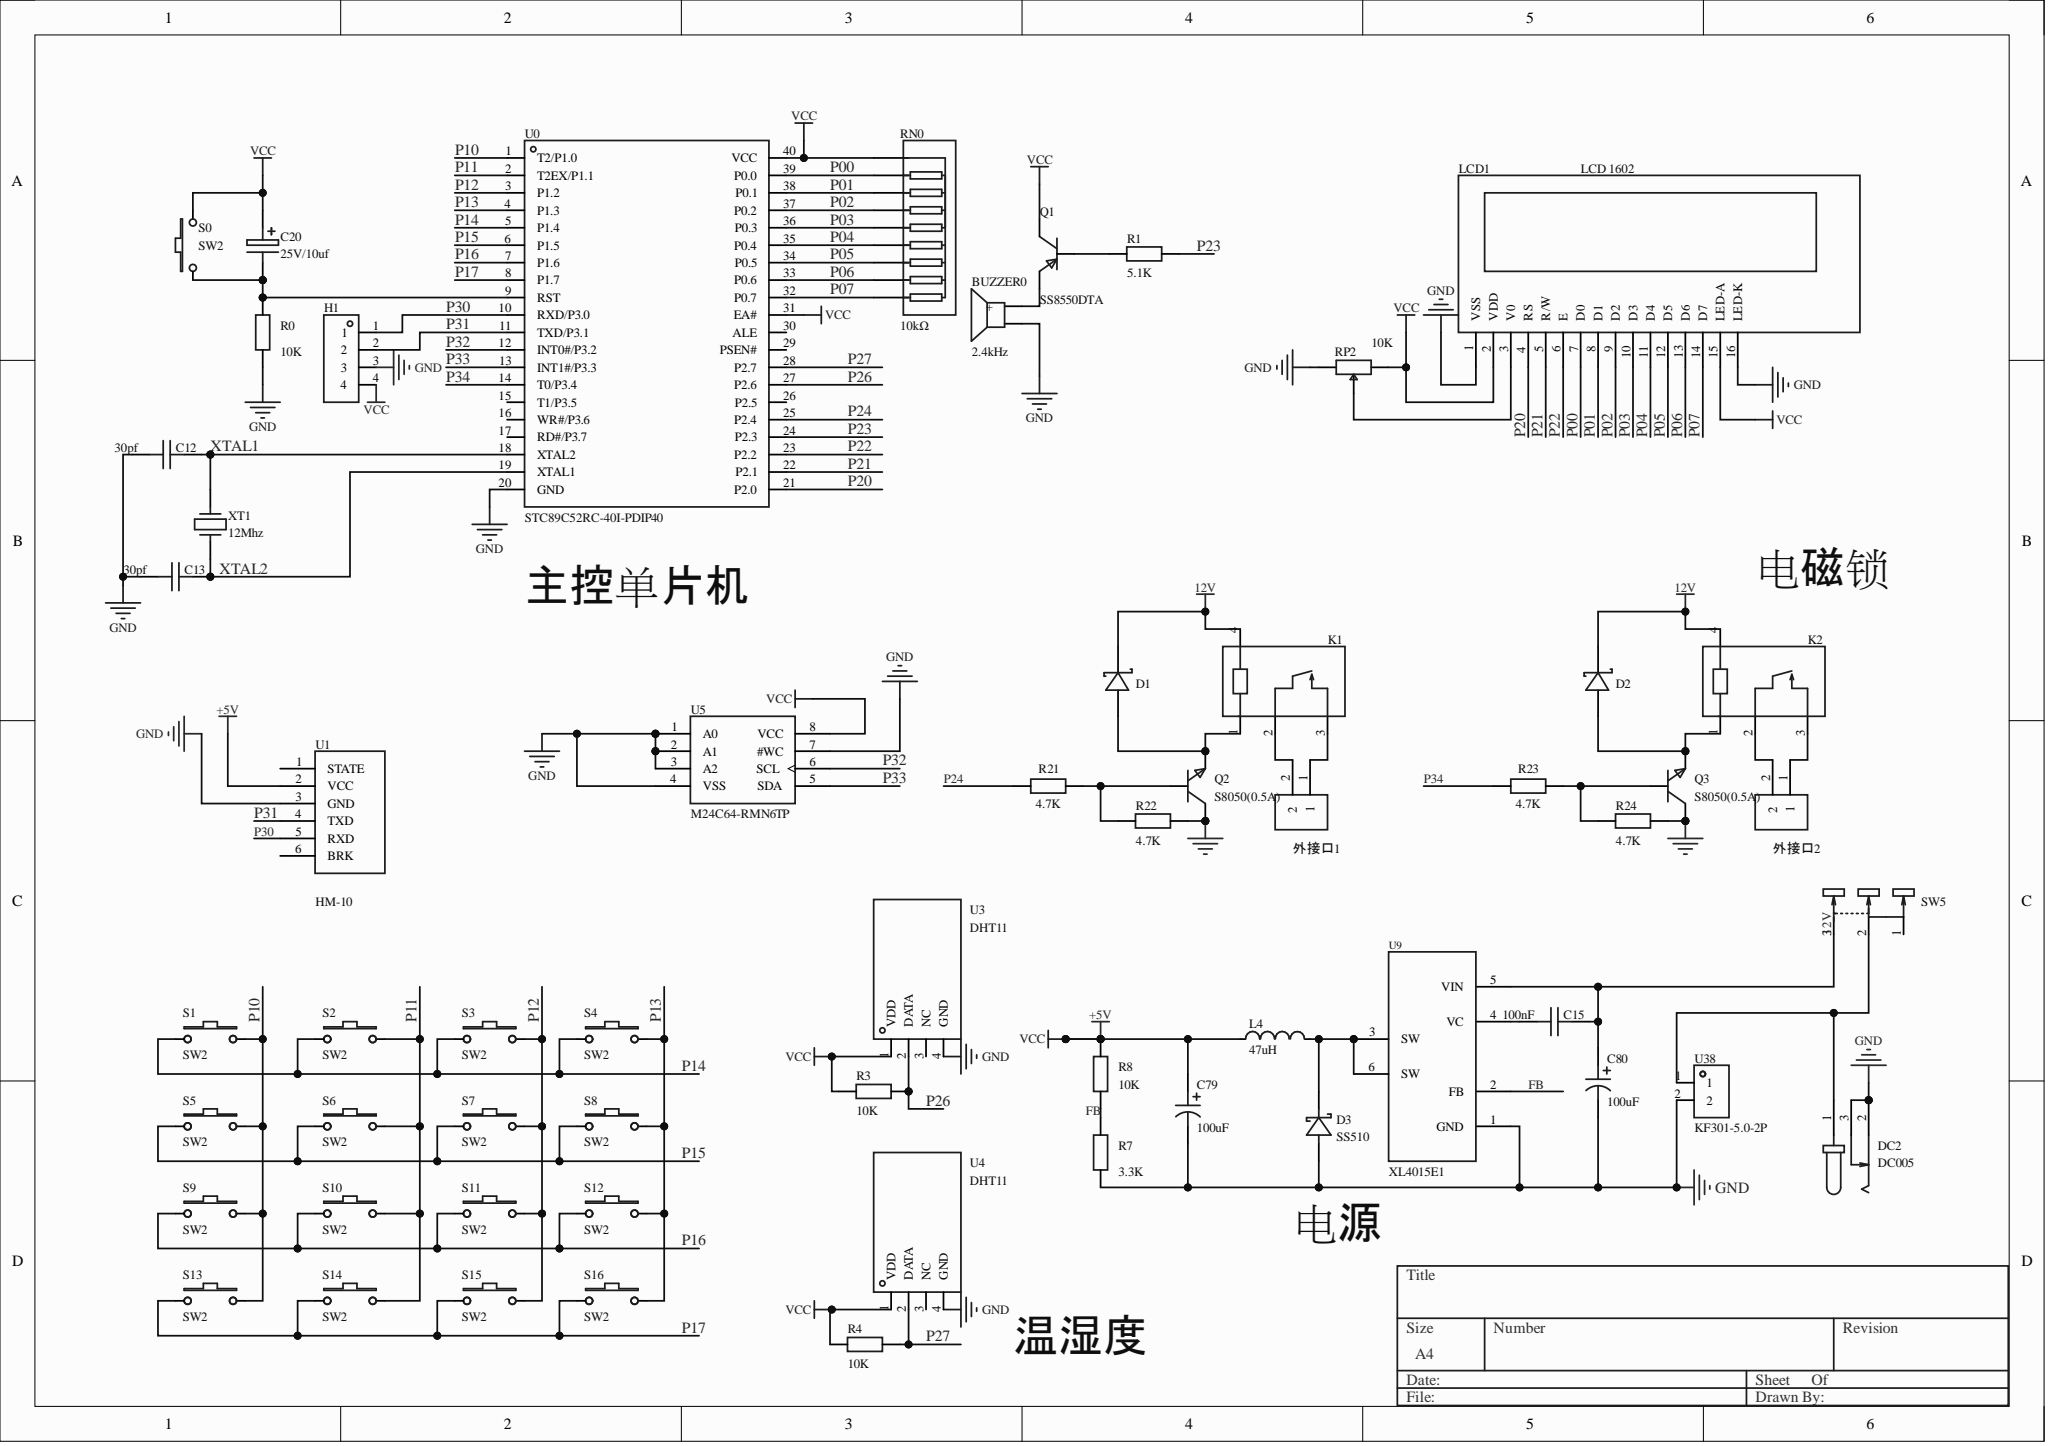Circuit board | Altium Designer | 59 parts | 49 nets
Bill of materials:
Comment,Description,Designator,Footprint,LibRef,Quantity
"2.4kHz","驱动方式:有源(内含驱动线路);构造类型:电磁式;额定电压:5V;频率:2.4kHz;声压(SPL):85dB;","BUZZER0","BUZ-TH_BD12.0-P7.60-D0.6-FD","TMB12A05_C96093","1"
"30pf","","C12, C13","C0805","CAP_0805","2"
"100nF","","C15","C0805","CAP_0805","1"
"CAP-E","","C20","CAP-TH_BD5.0-P2.00-D0.5-FD-A","CAP-E","1"
"100uF","容值:100uF;精度:±20%;额定电压:35V;纹波电流:87mA@120kHz;等效串联电阻:-;","C79, C80","CAP-SMD_BD6.3-L6.6-W6.6-LS7.4-FD","RVT100UF35V67RV0034","2"
"","","D1, D2","SMC_L6.9-W5.9-LS7.9-RD","SS34_C154551","2"
"SS510","二极管配置:独立式;直流反向耐压(Vr):100V;平均整流电流(Io):5A;正向压降(Vf):850mV@5A;","D3","SMA_L4.3-W2.6-LS5.0-RD","SS510_C727067","1"
"DC005","连接器类型:DC电源插座;安装方式:弯插;触点内径:2mm;触点外径:6.3mm;额定电流:500mA;额定电压:12V;工作温度:-30℃~+70℃;","DC2","DC-IN-TH_DC005","DC005","1"
"","","H1","HDR-TH_4P-P2.54-V-F","HDR-F_2.54_1x4P","1"
"","","K1, K2","RELAY-TH_G5NB-1A-E-DCXX","G5NB-1A-E-12VDC","2"
"47uH","类型:屏蔽电感;电感值:47uH;精度:±20%;额定电流:2.5A;饱和电流(Isat):4.6A;","L4","IND-SMD_L12.3-W12.3","SMDRI127-470MT","1"
"LCD 1602","LCD 1602","LCD1","LCD1602","LCD 1602","1"
"SS8550DTA","晶体管类型:PNP;集电极电流(Ic):1.5A;集射极击穿电压(Vceo):25V;耗散功率(Pd):2W;直流电流增益(hFE):40@800mA,1V;","Q1","TO-92-3_L4.8-W3.7-P2.54-L","SS8550DTA","1"
"S8050(0.5A)","晶体管类型:NPN;集电极电流(Ic):500mA;集射极击穿电压(Vceo):25V;耗散功率(Pd):300mW;直流电流增益(hFE):120;","Q2, Q3","SOT-23-3_L2.9-W1.3-P1.90-LS2.4-BR","S8050(0.5A)","2"
"10K","","R0, R3, R4, R8","R0805","Res_0805","4"
"5.1K","","R1","R0805","Res_0805","1"
"3.3K","","R7","R0805","Res_0805","1"
"4.7K","","R21, R22, R23, R24","R0805","Res_0805","4"
"10kΩ","","RN0","RES-ARRAY-TH_9P-P2.54-D1.0","A09-103JP","1"
"10K","","RP2","RES-ADJ-TH_3296W-1-203","10K","1"
"SW2","","S0, S1, S2, S3, S4, S5, S6, S7, S8, S9, S10, S11, S12, S13, S14, S15, S16","SW-SMD_L3.9-W2.9-LS5.0","SW2","17"
"SS-12D10L5","电路结构:单刀双掷;安装方式:直插;开关颜色:黑色;额定电流:3A;额定电压:125V;工作寿命:1万次;","SW5","SW-TH_SS-12D10L5","SS-12D10L5","1"
"STC89C52RC-40I-PDIP40","CPU内核:51家族;CPU最大主频:-;","U0","DIP-40_L52.0-W13.7-P2.54-LS15.2-BL","STC89C52RC-40I-PDIP40","1"
"HM-10","","U1","HM-10.288","hm10","1"
"DHT11","温度范围:-20℃~+60℃;湿度范围:5%RH~95%RH;湿度精度:±5%RH;","U3, U4","SENSOR-TH_DHT11","DHT11","2"
"M24C64-RMN6TP","接口类型:I2C;存储容量:64Kbit;时钟频率(fc):1MHz;","U5","SOIC-8_L5.0-W4.0-P1.27-LS6.0-BL","M24C64-RMN6TP","1"
"XL4015E1","功能类型:降压型;输入电压:-;输出电流(最大值):-;","U9","TO-263-5_L10.2-W8.9-P1.70-TL","XL4015E1","1"
"KF301-5.0-2P","结构:1x2P;间距:5mm;颜色:蓝色;安装方式:直插;额定电流:17A;额定电压:250V;排数:1;线规 - AWG:14~22;线规 - 平方毫米:1.5;每排PIN数:2;工作温度范围:-30℃~+120℃;","U38","CONN-TH_P5.00_KF301-5.0-2P","KF301-5.0-2P","1"
"XT","","XT1","HC-49S_L7.2-W3.2","XT","1"
"","","外接口1, 外接口2","CONN-TH_2P-P5.00_WJ500V-5.08-2P","WJ500V-5.08-2P","2"
Netlist (Protel format):
[
BUZZER0
BUZ-TH_BD12.0-P7.60-D0.6-FD
2.4kHz



]
[
C12
C0805
30pf



]
[
C13
C0805
30pf



]
[
C15
C0805
100nF



]
[
C20
CAP-TH_BD5.0-P2.00-D0.5-FD-A
CAP-E



]
[
C79
CAP-SMD_BD6.3-L6.6-W6.6-LS7.4-FD
100uF



]
[
C80
CAP-SMD_BD6.3-L6.6-W6.6-LS7.4-FD
100uF



]
[
D1
SMC_L6.9-W5.9-LS7.9-RD




]
[
D2
SMC_L6.9-W5.9-LS7.9-RD




]
[
D3
SMA_L4.3-W2.6-LS5.0-RD
SS510



]
[
DC2
DC-IN-TH_DC005
DC005



]
[
H1
HDR-TH_4P-P2.54-V-F




]
[
K1
RELAY-TH_G5NB-1A-E-DCXX




]
[
K2
RELAY-TH_G5NB-1A-E-DCXX




]
[
L4
IND-SMD_L12.3-W12.3
47uH



]
[
LCD1
LCD1602
LCD 1602



]
[
Q1
TO-92-3_L4.8-W3.7-P2.54-L
SS8550DTA



]
[
Q2
SOT-23-3_L2.9-W1.3-P1.90-LS2.4-BR
S8050(0.5A)



]
[
Q3
SOT-23-3_L2.9-W1.3-P1.90-LS2.4-BR
S8050(0.5A)



]
[
R0
R0805
10K



]
[
R1
R0805
5.1K



]
[
R3
R0805
10K



]
[
R4
R0805
10K



]
[
R7
R0805
3.3K



]
[
R8
R0805
10K



]
[
R21
R0805
4.7K



]
[
R22
R0805
4.7K



]
[
R23
R0805
4.7K



]
[
R24
R0805
4.7K



]
[
RN0
RES-ARRAY-TH_9P-P2.54-D1.0
10kΩ



]
[
RP2
RES-ADJ-TH_3296W-1-203
10K



]
[
S0
SW-SMD_L3.9-W2.9-LS5.0
SW2



]
[
S1
SW-SMD_L3.9-W2.9-LS5.0
SW2



]
[
S2
SW-SMD_L3.9-W2.9-LS5.0
SW2



]
[
S3
SW-SMD_L3.9-W2.9-LS5.0
SW2



]
[
S4
SW-SMD_L3.9-W2.9-LS5.0
SW2



]
[
S5
SW-SMD_L3.9-W2.9-LS5.0
SW2



]
[
S6
SW-SMD_L3.9-W2.9-LS5.0
SW2



]
[
S7
SW-SMD_L3.9-W2.9-LS5.0
SW2



]
[
S8
SW-SMD_L3.9-W2.9-LS5.0
SW2



]
[
S9
SW-SMD_L3.9-W2.9-LS5.0
SW2



]
[
S10
SW-SMD_L3.9-W2.9-LS5.0
SW2



]
[
S11
SW-SMD_L3.9-W2.9-LS5.0
SW2



]
[
S12
SW-SMD_L3.9-W2.9-LS5.0
SW2



]
[
S13
SW-SMD_L3.9-W2.9-LS5.0
SW2



]
[
S14
SW-SMD_L3.9-W2.9-LS5.0
SW2



]
[
S15
SW-SMD_L3.9-W2.9-LS5.0
SW2



]
[
S16
SW-SMD_L3.9-W2.9-LS5.0
SW2



]
[
SW5
SW-TH_SS-12D10L5
SS-12D10L5



]
[
U0
DIP-40_L52.0-W13.7-P2.54-LS15.2-BL
STC89C52RC-40I-PDIP40



]
[
U1
HM-10.288
HM-10



]
[
U3
SENSOR-TH_DHT11
DHT11



]
[
U4
SENSOR-TH_DHT11
DHT11



]
[
U5
SOIC-8_L5.0-W4.0-P1.27-LS6.0-BL
M24C64-RMN6TP



]
[
U9
TO-263-5_L10.2-W8.9-P1.70-TL
XL4015E1



]
[
U38
CONN-TH_P5.00_KF301-5.0-2P
KF301-5.0-2P



]
[
XT1
HC-49S_L7.2-W3.2
XT



]
[
外接口1
CONN-TH_2P-P5.00_WJ500V-5.08-2P




]
[
外接口2
CONN-TH_2P-P5.00_WJ500V-5.08-2P




]
(
XTAL2
C13-1
U0-19
XT1-1
)
(
XTAL1
C12-1
U0-18
XT1-2
)
(
P34
R23-2
U0-14
)
(
P33
U0-13
U5-5
)
(
P32
U0-12
U5-6
)
(
P31
H1-2
U0-11
U1-4
)
(
P30
H1-1
U0-10
U1-5
)
(
P27
R4-1
U0-28
U4-2
)
(
P26
R3-1
U0-27
U3-2
)
(
P24
R21-2
U0-25
)
(
P23
R1-1
U0-24
)
(
P22
LCD1-6
U0-23
)
(
P21
LCD1-5
U0-22
)
(
P20
LCD1-4
U0-21
)
(
P17
S13-1
S14-1
S15-1
S16-1
U0-8
)
(
P16
S9-1
S10-1
S11-1
S12-1
U0-7
)
(
P15
S5-1
S6-1
S7-1
S8-1
U0-6
)
(
P14
S1-1
S2-1
S3-1
S4-1
U0-5
)
(
P13
S4-2
S8-2
S12-2
S16-2
U0-4
)
(
P12
S3-2
S7-2
S11-2
S15-2
U0-3
)
(
P11
S2-2
S6-2
S10-2
S14-2
U0-2
)
(
P10
S1-2
S5-2
S9-2
S13-2
U0-1
)
(
P07
LCD1-14
RN0-9
U0-32
)
(
P06
LCD1-13
RN0-8
U0-33
)
(
P05
LCD1-12
RN0-7
U0-34
)
(
P04
LCD1-11
RN0-6
U0-35
)
(
P03
LCD1-10
RN0-5
U0-36
)
(
P02
LCD1-9
RN0-4
U0-37
)
(
P01
LCD1-8
RN0-3
U0-38
)
(
P00
LCD1-7
RN0-2
U0-39
)
(
NetQ3_1
Q3-1
R23-1
R24-2
)
(
NetQ2_1
Q2-1
R21-1
R22-2
)
(
NetQ1_2
Q1-2
R1-2
)
(
NetLCD1_3
LCD1-3
RP2-2
)
(
NetK2_3
K2-3
外接口2-1
)
(
NetK2_2
K2-2
外接口2-2
)
(
NetK1_3
K1-3
外接口1-1
)
(
NetK1_2
K1-2
外接口1-2
)
(
NetDC2_1
DC2-1
SW5-2
U38-1
)
(
NetD3_1
D3-1
L4-2
U9-3
U9-6
)
(
NetD2_2
D2-2
K2-1
Q3-2
)
(
NetD1_2
D1-2
K1-1
Q2-2
)
(
NetC20_2
C20-2
R0-2
S0-1
U0-9
)
(
NetC15_2
C15-2
U9-4
)
(
NetBUZZER0_1
BUZZER0-1
Q1-1
)
(
GND
BUZZER0-2
C12-2
C13-2
C79-2
C80-2
D3-2
DC2-2
DC2-3
H1-3
LCD1-1
LCD1-16
Q2-3
Q3-3
R0-1
R7-1
R22-1
R24-1
RP2-3
U0-20
U1-3
U3-4
U4-4
U5-1
U5-2
U5-3
U5-4
U5-7
U9-1
U38-2
)
(
FB
R7-2
R8-1
U9-2
)
(
+5V
C20-1
C79-1
H1-4
L4-1
LCD1-2
LCD1-15
Q1-3
R3-2
R4-2
R8-2
RN0-1
RP2-1
S0-2
U0-31
U0-40
U1-2
U3-1
U4-1
U5-8
)
(
12V
C15-1
C80-1
D1-1
D2-1
K1-4
K2-4
SW5-3
U9-5
)